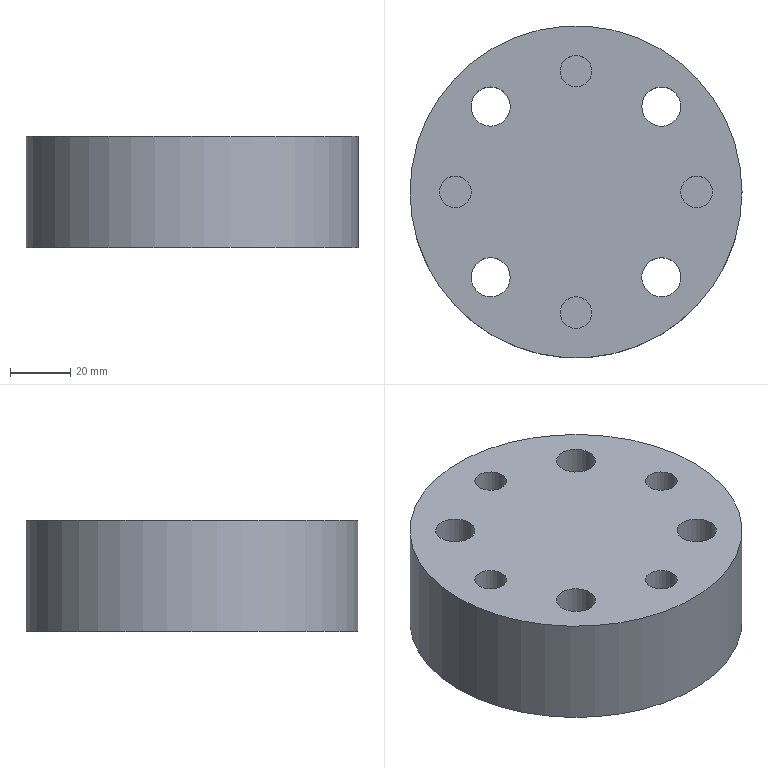CAM job | NX | 3-axis milling, drilling | part box 110 x 110 x 37 mm | stock box 110 x 110 x 37 mm
Tools:
number,name,description,diameter,corner_radius,flute_length,length,flutes
1,ZXZ,Milling Tool-5 Parameters,6.0,0.0,50.0,75.0,2
3,13.0ZT,Drilling Tool,13.0,0.0,35.0,50.0,2
4,D6A45,Milling Tool-5 Parameters,6.0,0.0,50.0,75.0,2
2,10.5ZT,Drilling Tool,10.5,0.0,35.0,50.0,2
Operations:
program,operation,operation_type,tool,method,geometry_group,spindle_rpm,surface_speed,feed_per_tooth,feed_cut,feed_plunge,cut_length_mm,path_length_mm,cut_time_min,machine_time_min
1,DRILLING,Operation,ZXZ,METHOD,A,3000.0,0.0,0.0,250.0,0.0,32.0,360.329,0.128,0.1608
1,DRILLING_COPY,Operation,13.0ZT,METHOD,A,800.0,32.0,0.0625,100.0,0.0,177.622,594.189,1.776,1.818
1,DRILLING_COPY_COPY,Operation,10.5ZT,METHOD,A,800.0,32.0,0.0625,100.0,0.0,104.618,448.18,1.046,1.081
1,PLANAR_MILL,PlanarMilling,D6A45,METHOD,A,7500.0,141.0,0.0833,1250.0,100.0,333.315,998.327,0.2667,0.3332